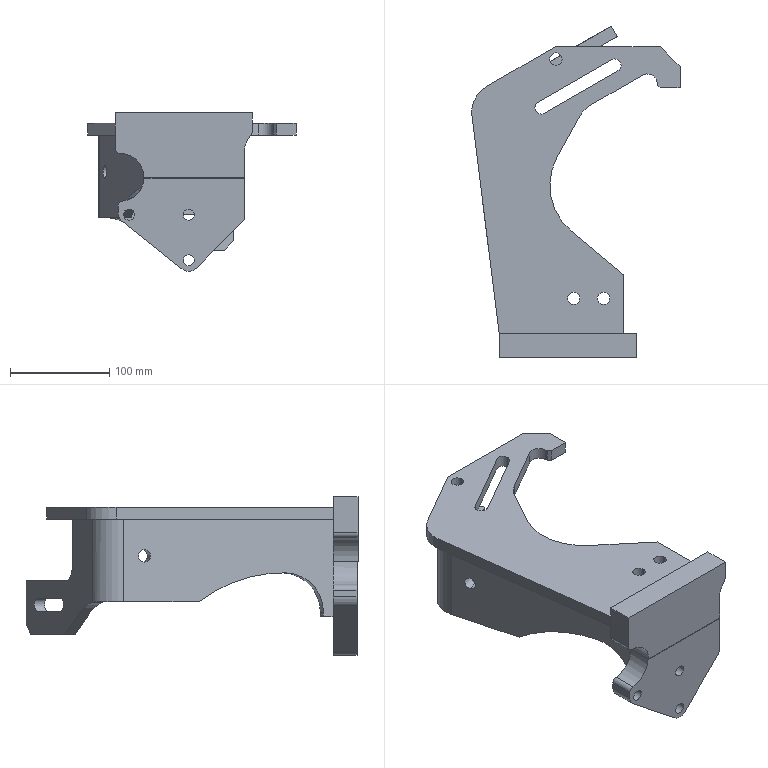Part | SolidWorks | features BaseBody 3 | 3 solids | 88 faces | box 209.597 x 333.937 x 159.51 mm | volume 1061009 mm3 | plane 49 | cylinder 38 | spline 1 | commonest cylinder face diameters 12.5 x8 11 x6 10 x3 13 x3 13.3 x2 22 x2